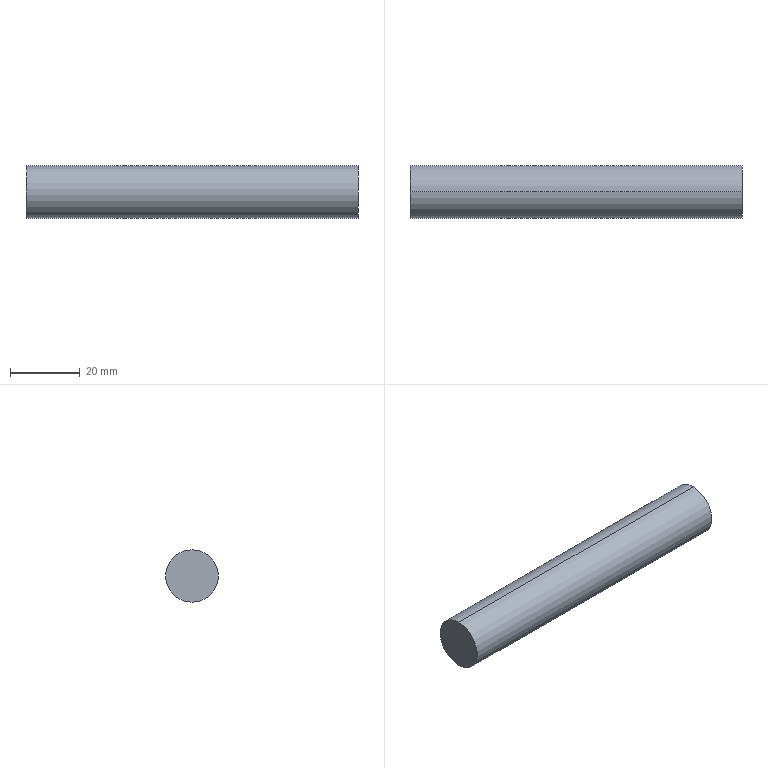Part | NX | features BREP 1 | 1 solid | 4 faces | box 95 x 15 x 15 mm | volume 16788 mm3 | cylinder 2 | plane 2 | commonest cylinder face diameters 15 x2
STEP:
#1=CARTESIAN_POINT('',(47.5,-3.75,7.5));
#2=VERTEX_POINT('',#1);
#3=CARTESIAN_POINT('',(47.5,-3.75,-7.5));
#4=VERTEX_POINT('',#3);
#5=CARTESIAN_POINT('',(47.5,-3.75,0.));
#6=DIRECTION('',(-1.,0.,0.));
#7=DIRECTION('',(0.,0.,1.));
#8=AXIS2_PLACEMENT_3D('',#5,#6,#7);
#9=CIRCLE('',#8,7.5);
#10=EDGE_CURVE('',#2,#4,#9,.T.);
#11=ORIENTED_EDGE('',*,*,#10,.T.);
#12=CARTESIAN_POINT('',(-47.5,-3.75,-7.5));
#13=VERTEX_POINT('',#12);
#14=CARTESIAN_POINT('',(-47.5,-3.75,-7.5));
#15=DIRECTION('',(-1.,0.,0.));
#16=VECTOR('',#15,1000.);
#17=LINE('',#14,#16);
#18=EDGE_CURVE('',#4,#13,#17,.T.);
#19=ORIENTED_EDGE('',*,*,#18,.T.);
#20=CARTESIAN_POINT('',(-47.5,-3.75,7.5));
#21=VERTEX_POINT('',#20);
#22=CARTESIAN_POINT('',(-47.5,-3.75,0.));
#23=DIRECTION('',(-1.,0.,0.));
#24=DIRECTION('',(0.,0.,1.));
#25=AXIS2_PLACEMENT_3D('',#22,#23,#24);
#26=CIRCLE('',#25,7.5);
#27=EDGE_CURVE('',#21,#13,#26,.T.);
#28=ORIENTED_EDGE('',*,*,#27,.F.);
#29=CARTESIAN_POINT('',(-47.5,-3.75,7.5));
#30=DIRECTION('',(-1.,0.,0.));
#31=VECTOR('',#30,1000.);
#32=LINE('',#29,#31);
#33=EDGE_CURVE('',#2,#21,#32,.T.);
#34=ORIENTED_EDGE('',*,*,#33,.F.);
#35=EDGE_LOOP('',(#11,#19,#28,#34));
#36=FACE_BOUND('',#35,.T.);
#37=CARTESIAN_POINT('',(-47.5,-3.75,0.));
#38=DIRECTION('',(-1.,0.,0.));
#39=DIRECTION('',(0.,0.,-1.));
#40=AXIS2_PLACEMENT_3D('',#37,#38,#39);
#41=CYLINDRICAL_SURFACE('',#40,7.5);
#42=ADVANCED_FACE('',(#36),#41,.T.);
#43=ORIENTED_EDGE('',*,*,#10,.F.);
#44=CARTESIAN_POINT('',(47.5,-3.75,0.));
#45=DIRECTION('',(-1.,0.,0.));
#46=DIRECTION('',(0.,0.,1.));
#47=AXIS2_PLACEMENT_3D('',#44,#45,#46);
#48=CIRCLE('',#47,7.5);
#49=EDGE_CURVE('',#4,#2,#48,.T.);
#50=ORIENTED_EDGE('',*,*,#49,.F.);
#51=EDGE_LOOP('',(#43,#50));
#52=FACE_BOUND('',#51,.T.);
#53=CARTESIAN_POINT('',(47.5,-3.75,0.));
#54=DIRECTION('',(-1.,0.,0.));
#55=DIRECTION('',(0.,0.,-1.));
#56=AXIS2_PLACEMENT_3D('',#53,#54,#55);
#57=PLANE('',#56);
#58=ADVANCED_FACE('',(#52),#57,.F.);
#59=ORIENTED_EDGE('',*,*,#27,.T.);
#60=CARTESIAN_POINT('',(-47.5,-3.75,0.));
#61=DIRECTION('',(-1.,0.,0.));
#62=DIRECTION('',(0.,0.,1.));
#63=AXIS2_PLACEMENT_3D('',#60,#61,#62);
#64=CIRCLE('',#63,7.5);
#65=EDGE_CURVE('',#13,#21,#64,.T.);
#66=ORIENTED_EDGE('',*,*,#65,.T.);
#67=EDGE_LOOP('',(#59,#66));
#68=FACE_BOUND('',#67,.T.);
#69=CARTESIAN_POINT('',(-47.5,-3.75,0.));
#70=DIRECTION('',(1.,0.,0.));
#71=DIRECTION('',(0.,-1.,0.));
#72=AXIS2_PLACEMENT_3D('',#69,#70,#71);
#73=PLANE('',#72);
#74=ADVANCED_FACE('',(#68),#73,.F.);
#75=ORIENTED_EDGE('',*,*,#18,.F.);
#76=ORIENTED_EDGE('',*,*,#49,.T.);
#77=ORIENTED_EDGE('',*,*,#33,.T.);
#78=ORIENTED_EDGE('',*,*,#65,.F.);
#79=EDGE_LOOP('',(#75,#76,#77,#78));
#80=FACE_BOUND('',#79,.T.);
#81=CARTESIAN_POINT('',(-47.5,-3.75,0.));
#82=DIRECTION('',(-1.,0.,0.));
#83=DIRECTION('',(0.,0.,-1.));
#84=AXIS2_PLACEMENT_3D('',#81,#82,#83);
#85=CYLINDRICAL_SURFACE('',#84,7.5);
#86=ADVANCED_FACE('',(#80),#85,.T.);
#87=CLOSED_SHELL('',(#42,#58,#74,#86));
#88=MANIFOLD_SOLID_BREP('',#87);
#89=(LENGTH_UNIT()NAMED_UNIT(*)SI_UNIT(.MILLI.,.METRE.));
#90=UNCERTAINTY_MEASURE_WITH_UNIT(LENGTH_MEASURE(0.00001),#89,'','');
#91=(NAMED_UNIT(*)PLANE_ANGLE_UNIT()SI_UNIT($,.RADIAN.));
#92=(NAMED_UNIT(*)SI_UNIT($,.STERADIAN.)SOLID_ANGLE_UNIT());
#93=(GEOMETRIC_REPRESENTATION_CONTEXT(3)GLOBAL_UNCERTAINTY_ASSIGNED_CONTEXT((#90))GLOBAL_UNIT_ASSIGNED_CONTEXT((#89,#91,#92))REPRESENTATION_CONTEXT('',''));
#94=ADVANCED_BREP_SHAPE_REPRESENTATION('',(#88),#93);